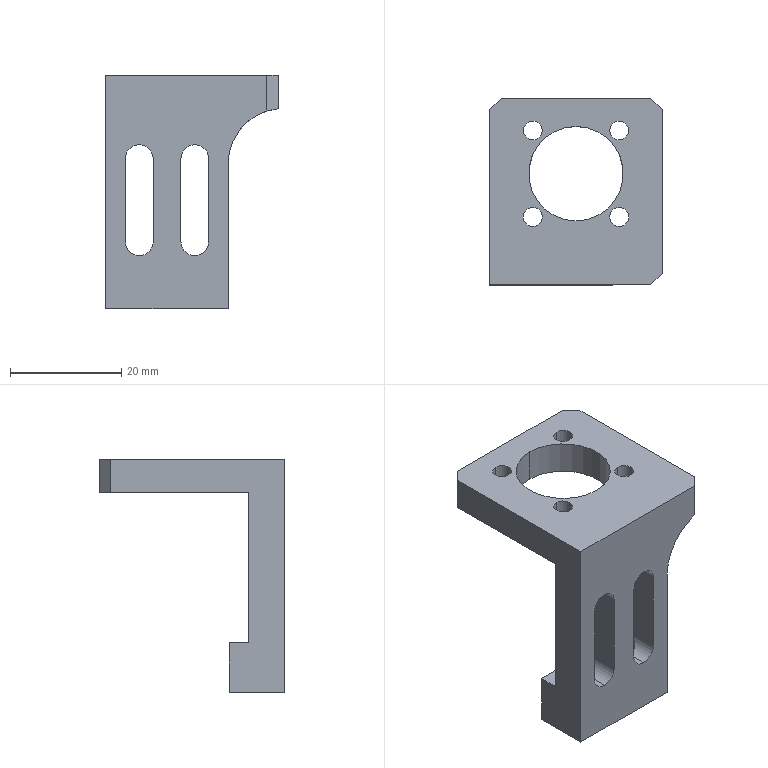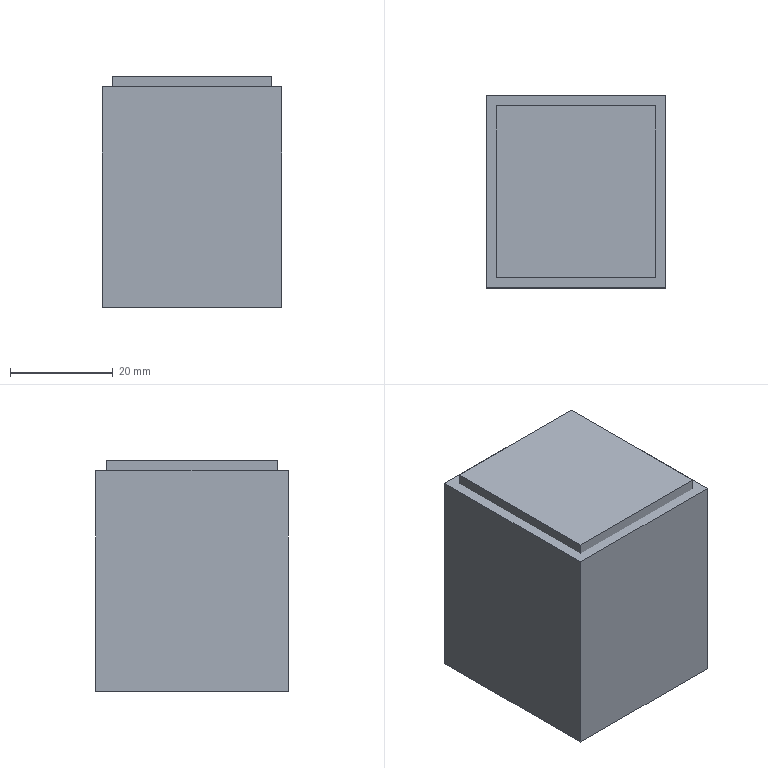CAM job | NX | 3+2 milling, drilling | part box 31 x 33.478 x 42 mm | stock box 35 x 37.478 x 45 mm
Tools:
number,name,description,diameter,corner_radius,flute_length,length,flutes
19,D80,Milling Tool-5 Parameters,80.0,0.0,50.0,75.0,2
15,D10,Milling Tool-5 Parameters,10.0,0.0,50.0,75.0,2
14,D10JING,Milling Tool-5 Parameters,10.0,0.0,50.0,75.0,2
1,D6A45,Milling Tool-5 Parameters,6.0,0.0,50.0,75.0,2
2,2.5ZT,Drilling Tool,2.0,0.0,35.0,50.0,2
16,3.4ZT,Drilling Tool,3.4,0.0,35.0,50.0,2
11,D4,Milling Tool-5 Parameters,4.0,0.0,50.0,75.0,2
Operations:
program,operation,operation_type,tool,method,geometry_group,spindle_rpm,surface_speed,feed_per_tooth,feed_cut,feed_plunge,cut_length_mm,path_length_mm,cut_time_min,machine_time_min
1,FLOOR_WALL,VolumeBased25DMillingOperation,D80,METHOD,A,6500.0,1633.0,0.1154,1500.0,100.0,127.0,181.0,0.0847,0.0901
1,DRILLING,Operation,D6A45,METHOD,A,9500.0,179.0,0.0132,250.0,0.0,20.0,166.489,0.08,0.0946
1,DRILLING_COPY_COPY_COPY,Operation,3.4ZT,METHOD,A,2000.0,21.0,0.05,200.0,0.0,46.086,208.701,0.2304,0.2467
1,ZLEVEL_PROFILE,ZLevelMilling,D10,METHOD,A,9500.0,298.0,0.1579,3000.0,1000.0,6820.764,6919.764,2.305,2.315
1,ZLEVEL_PROFILE_1,ZLevelMilling,D10JING,METHOD,A,9500.0,298.0,0.0789,1500.0,1000.0,637.007,750.007,0.426,0.4373
1,HOLE_MILLING,CylinderMilling,D10JING,METHOD,A,9500.0,298.0,0.0789,1500.0,100.0,271.313,336.813,0.1809,0.1874
1,PLANAR_MILL_COPY,PlanarMilling,D6A45,METHOD,A,9500.0,179.0,0.0658,1250.0,100.0,225.333,649.443,0.1803,0.2227
2,FLOOR_WALL_COPY,VolumeBased25DMillingOperation,D80,METHOD,B,6500.0,1633.0,0.1154,1500.0,100.0,369.0,759.001,0.246,0.285
2,DRILLING_COPY,Operation,D6A45,METHOD,B,9500.0,179.0,0.0132,250.0,0.0,8.0,91.369,0.032,0.0403
2,DRILLING_COPY_COPY_COPY_1,Operation,2.5ZT,METHOD,B,2000.0,12.0,0.025,100.0,0.0,32.022,139.414,0.3202,0.331
2,PLANAR_MILL_COPY_COPY,PlanarMilling,D6A45,METHOD,B,9500.0,179.0,0.0658,1250.0,800.0,87.242,280.365,0.0728,0.0921
3,ZLEVEL_PROFILE_COPY,ZLevelMilling,D10,METHOD,C,9500.0,298.0,0.1579,3000.0,1000.0,537.292,607.292,0.1819,0.1889
3,ZLEVEL_PROFILE_COPY_COPY,ZLevelMilling,D10JING,METHOD,C,9500.0,298.0,0.0789,1500.0,1000.0,41.522,122.522,0.029,0.0371
3,ZLEVEL_PROFILE_COPY_1,ZLevelMilling,D4,METHOD,C,9500.0,119.0,0.0868,1650.0,1000.0,1330.348,1469.469,0.8346,0.8485
3,PLANAR_MILL_COPY_COPY_1,PlanarMilling,D6A45,METHOD,C,9500.0,179.0,0.0658,1250.0,100.0,242.8,442.645,0.1942,0.2142
3,PLANAR_MILL_COPY_COPY_1_COPY,PlanarMilling,D6A45,METHOD,C,9500.0,179.0,0.0658,1250.0,100.0,11.505,73.505,0.0092,0.0154
4,FLOOR_WALL_1,VolumeBased25DMillingOperation,D10,METHOD,D,9500.0,298.0,0.1579,3000.0,1000.0,4823.701,4998.025,1.616,1.633
4,FLOOR_WALL_1_COPY,VolumeBased25DMillingOperation,D10,METHOD,D,9500.0,298.0,0.1579,3000.0,1000.0,984.087,1091.844,0.3327,0.3434
4,FLOOR_WALL_1_COPY_COPY,VolumeBased25DMillingOperation,D10JING,METHOD,D,9500.0,298.0,0.0789,1500.0,1000.0,412.717,678.887,0.2854,0.312
4,FLOOR_WALL_1_COPY_COPY_COPY,VolumeBased25DMillingOperation,D10JING,METHOD,D,9500.0,298.0,0.0789,1500.0,1000.0,185.91,423.78,0.1322,0.156
4,PLANAR_MILL_COPY_COPY_1_COPY_1,PlanarMilling,D6A45,METHOD,D,9500.0,179.0,0.0658,1250.0,100.0,72.749,178.706,0.0582,0.0688
4,PLANAR_MILL_COPY_COPY_1_COPY_1_COPY,PlanarMilling,D6A45,METHOD,D,9500.0,179.0,0.0658,1250.0,100.0,135.445,632.452,0.1084,0.1581